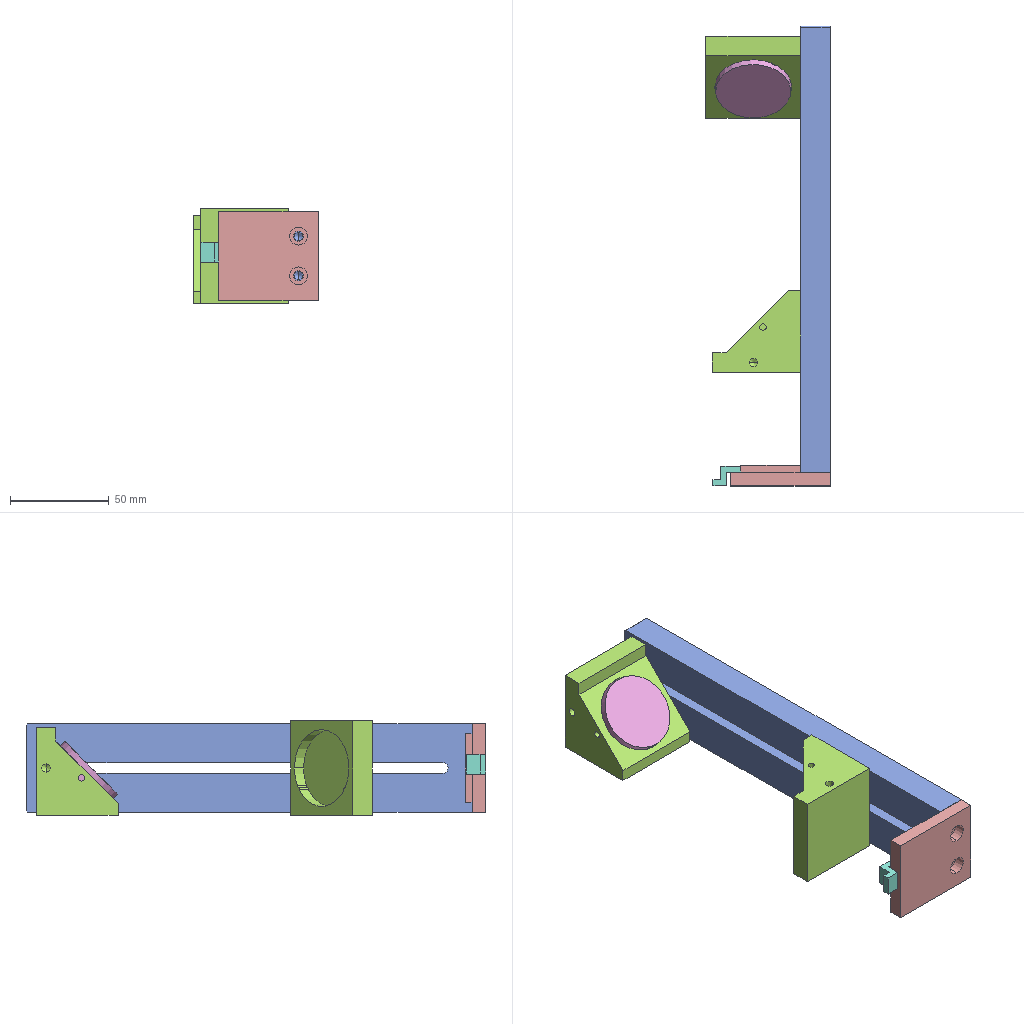Assembly | SolidWorks | 8 different items | 10 placed | box 63 x 233 x 48 mm
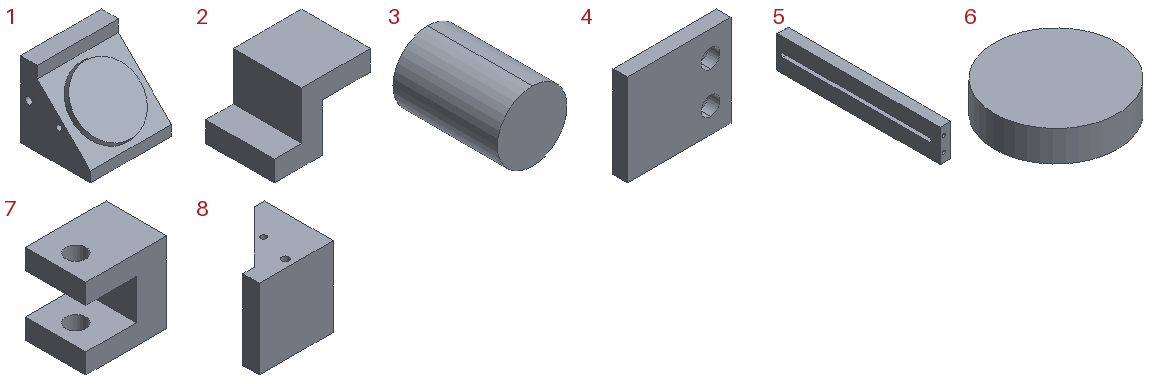Parts list (item | name | quantity | size | volume | features):
1 | (subassembly) | x1 | 48 x 41.5 x 44.63 mm | 57174 mm3 | -
2 | - | x1 | 14 x 10 x 10 mm | 630 mm3 | features Extrusion 1
3 | - | x1 | 20 x 30 x 20 mm | 9425 mm3 | features Extrusion 1
4 | - | x1 | 50.4 x 10.4 x 44.6 mm | 18550 mm3 | features MoveFace 4, ICE 2, Cut 1, DelFace 1, SplitBody 1
5 | - | x1 | 15 x 226 x 44.6 mm | 129976 mm3 | features MoveFace 6, ICE 2, HoleWzd 1, SplitBody 1
6 | - | x2 | 38.1 x 38.1 x 9.525 mm | 10859 mm3 | features Extrusion 1
7 | - | x1 | 40 x 30 x 40 mm | 31429 mm3 | features Extrusion 1, ICE 1
8 | - | x2 | 44.63 x 41.5 x 48 mm | 46315 mm3 | features ICE 7, HoleWzd 3, MoveFace 2, Extrusion 1, Fillet 1, MirrorPattern 1
Mates (type | each side: item.copy, entity, surface, feature):
Coincident | 4.1 face plane Base part body-1 | 2.1 face plane Boss-Extrude1 | 2 times